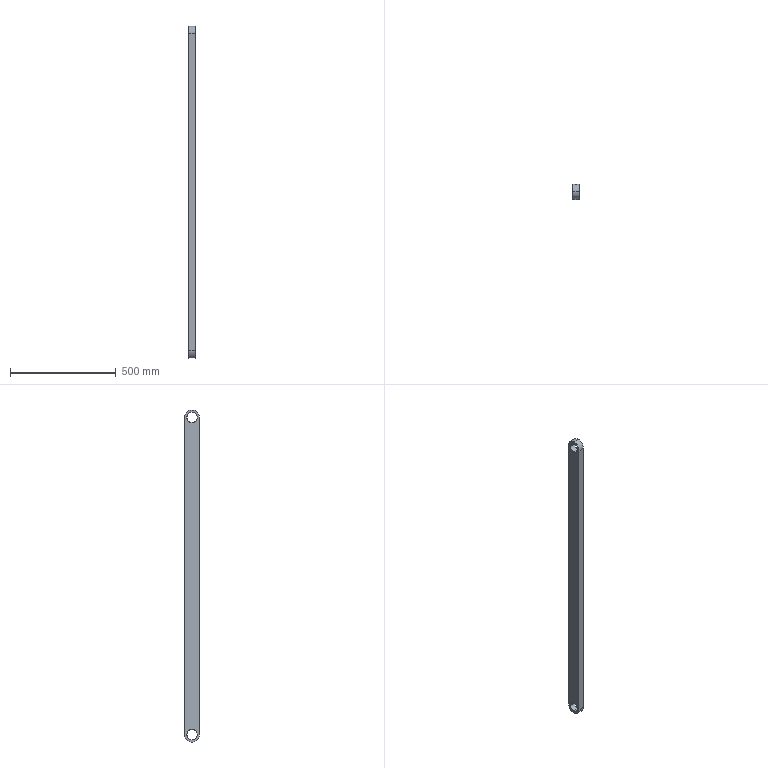Part | SolidWorks | features Chamfer 1, Extrusion 1, HoleWzd 1 | 1 solid | 23 faces | box 30 x 70 x 1570 mm | volume 3155166 mm3 | cylinder 11 | cone 8 | plane 4 | commonest cylinder face diameters 9 x4 48 x4 70 x3
STEP:
#1=CARTESIAN_POINT('',(14.,0.,774.));
#2=VERTEX_POINT('',#1);
#3=CARTESIAN_POINT('',(14.,0.,726.));
#4=VERTEX_POINT('',#3);
#5=CARTESIAN_POINT('',(14.,0.,750.));
#6=DIRECTION('',(1.,0.,0.));
#7=DIRECTION('',(0.,0.,-1.));
#8=AXIS2_PLACEMENT_3D('',#5,#6,#7);
#9=CIRCLE('',#8,24.);
#10=EDGE_CURVE('',#2,#4,#9,.T.);
#11=ORIENTED_EDGE('',*,*,#10,.F.);
#12=CARTESIAN_POINT('',(15.,0.,775.));
#13=VERTEX_POINT('',#12);
#14=CARTESIAN_POINT('',(14.,0.,774.));
#15=DIRECTION('',(0.7071,0.,0.7071));
#16=VECTOR('',#15,1000.);
#17=LINE('',#14,#16);
#18=EDGE_CURVE('',#2,#13,#17,.T.);
#19=ORIENTED_EDGE('',*,*,#18,.T.);
#20=CARTESIAN_POINT('',(15.,0.,725.));
#21=VERTEX_POINT('',#20);
#22=CARTESIAN_POINT('',(15.,0.,750.));
#23=DIRECTION('',(-1.,0.,0.));
#24=DIRECTION('',(0.,0.,-1.));
#25=AXIS2_PLACEMENT_3D('',#22,#23,#24);
#26=CIRCLE('',#25,25.);
#27=EDGE_CURVE('',#21,#13,#26,.T.);
#28=ORIENTED_EDGE('',*,*,#27,.F.);
#29=CARTESIAN_POINT('',(14.,0.,726.));
#30=DIRECTION('',(0.7071,0.,-0.7071));
#31=VECTOR('',#30,1000.);
#32=LINE('',#29,#31);
#33=EDGE_CURVE('',#4,#21,#32,.T.);
#34=ORIENTED_EDGE('',*,*,#33,.F.);
#35=EDGE_LOOP('',(#11,#19,#28,#34));
#36=FACE_OUTER_BOUND('',#35,.T.);
#37=CARTESIAN_POINT('',(14.,0.,750.));
#38=DIRECTION('',(1.,0.,0.));
#39=DIRECTION('',(0.,0.,-1.));
#40=AXIS2_PLACEMENT_3D('',#37,#38,#39);
#41=CONICAL_SURFACE('',#40,24.,0.7854);
#42=ADVANCED_FACE('',(#36),#41,.F.);
#43=CARTESIAN_POINT('',(-14.,0.,726.));
#44=VERTEX_POINT('',#43);
#45=CARTESIAN_POINT('',(-14.,0.,774.));
#46=VERTEX_POINT('',#45);
#47=CARTESIAN_POINT('',(-14.,0.,750.));
#48=DIRECTION('',(-1.,0.,0.));
#49=DIRECTION('',(0.,0.,-1.));
#50=AXIS2_PLACEMENT_3D('',#47,#48,#49);
#51=CIRCLE('',#50,24.);
#52=EDGE_CURVE('',#44,#46,#51,.T.);
#53=ORIENTED_EDGE('',*,*,#52,.F.);
#54=CARTESIAN_POINT('',(-15.,0.,725.));
#55=VERTEX_POINT('',#54);
#56=CARTESIAN_POINT('',(-15.,0.,725.));
#57=DIRECTION('',(-0.7071,0.,-0.7071));
#58=VECTOR('',#57,1000.);
#59=LINE('',#56,#58);
#60=EDGE_CURVE('',#44,#55,#59,.T.);
#61=ORIENTED_EDGE('',*,*,#60,.T.);
#62=CARTESIAN_POINT('',(-15.,0.,775.));
#63=VERTEX_POINT('',#62);
#64=CARTESIAN_POINT('',(-15.,0.,750.));
#65=DIRECTION('',(1.,0.,0.));
#66=DIRECTION('',(0.,0.,-1.));
#67=AXIS2_PLACEMENT_3D('',#64,#65,#66);
#68=CIRCLE('',#67,25.);
#69=EDGE_CURVE('',#63,#55,#68,.T.);
#70=ORIENTED_EDGE('',*,*,#69,.F.);
#71=CARTESIAN_POINT('',(-15.,0.,775.));
#72=DIRECTION('',(-0.7071,0.,0.7071));
#73=VECTOR('',#72,1000.);
#74=LINE('',#71,#73);
#75=EDGE_CURVE('',#46,#63,#74,.T.);
#76=ORIENTED_EDGE('',*,*,#75,.F.);
#77=EDGE_LOOP('',(#53,#61,#70,#76));
#78=FACE_OUTER_BOUND('',#77,.T.);
#79=CARTESIAN_POINT('',(-15.,0.,750.));
#80=DIRECTION('',(-1.,0.,0.));
#81=DIRECTION('',(0.,0.,1.));
#82=AXIS2_PLACEMENT_3D('',#79,#80,#81);
#83=CONICAL_SURFACE('',#82,25.,0.7854);
#84=ADVANCED_FACE('',(#78),#83,.F.);
#85=CARTESIAN_POINT('',(-14.,0.,-774.));
#86=VERTEX_POINT('',#85);
#87=CARTESIAN_POINT('',(-14.,0.,-726.));
#88=VERTEX_POINT('',#87);
#89=CARTESIAN_POINT('',(-14.,0.,-750.));
#90=DIRECTION('',(-1.,0.,0.));
#91=DIRECTION('',(0.,0.,-1.));
#92=AXIS2_PLACEMENT_3D('',#89,#90,#91);
#93=CIRCLE('',#92,24.);
#94=EDGE_CURVE('',#86,#88,#93,.T.);
#95=ORIENTED_EDGE('',*,*,#94,.F.);
#96=CARTESIAN_POINT('',(-15.,0.,-775.));
#97=VERTEX_POINT('',#96);
#98=CARTESIAN_POINT('',(-15.,0.,-775.));
#99=DIRECTION('',(-0.7071,0.,-0.7071));
#100=VECTOR('',#99,1000.);
#101=LINE('',#98,#100);
#102=EDGE_CURVE('',#86,#97,#101,.T.);
#103=ORIENTED_EDGE('',*,*,#102,.T.);
#104=CARTESIAN_POINT('',(-15.,0.,-725.));
#105=VERTEX_POINT('',#104);
#106=CARTESIAN_POINT('',(-15.,0.,-750.));
#107=DIRECTION('',(1.,0.,0.));
#108=DIRECTION('',(0.,0.,-1.));
#109=AXIS2_PLACEMENT_3D('',#106,#107,#108);
#110=CIRCLE('',#109,25.);
#111=EDGE_CURVE('',#105,#97,#110,.T.);
#112=ORIENTED_EDGE('',*,*,#111,.F.);
#113=CARTESIAN_POINT('',(-15.,0.,-725.));
#114=DIRECTION('',(-0.7071,0.,0.7071));
#115=VECTOR('',#114,1000.);
#116=LINE('',#113,#115);
#117=EDGE_CURVE('',#88,#105,#116,.T.);
#118=ORIENTED_EDGE('',*,*,#117,.F.);
#119=EDGE_LOOP('',(#95,#103,#112,#118));
#120=FACE_OUTER_BOUND('',#119,.T.);
#121=CARTESIAN_POINT('',(-15.,0.,-750.));
#122=DIRECTION('',(-1.,0.,0.));
#123=DIRECTION('',(0.,0.,1.));
#124=AXIS2_PLACEMENT_3D('',#121,#122,#123);
#125=CONICAL_SURFACE('',#124,25.,0.7854);
#126=ADVANCED_FACE('',(#120),#125,.F.);
#127=CARTESIAN_POINT('',(14.,0.,-726.));
#128=VERTEX_POINT('',#127);
#129=CARTESIAN_POINT('',(14.,0.,-774.));
#130=VERTEX_POINT('',#129);
#131=CARTESIAN_POINT('',(14.,0.,-750.));
#132=DIRECTION('',(1.,0.,0.));
#133=DIRECTION('',(0.,0.,-1.));
#134=AXIS2_PLACEMENT_3D('',#131,#132,#133);
#135=CIRCLE('',#134,24.);
#136=EDGE_CURVE('',#128,#130,#135,.T.);
#137=ORIENTED_EDGE('',*,*,#136,.F.);
#138=CARTESIAN_POINT('',(15.,0.,-725.));
#139=VERTEX_POINT('',#138);
#140=CARTESIAN_POINT('',(14.,0.,-726.));
#141=DIRECTION('',(0.7071,0.,0.7071));
#142=VECTOR('',#141,1000.);
#143=LINE('',#140,#142);
#144=EDGE_CURVE('',#128,#139,#143,.T.);
#145=ORIENTED_EDGE('',*,*,#144,.T.);
#146=CARTESIAN_POINT('',(15.,0.,-775.));
#147=VERTEX_POINT('',#146);
#148=CARTESIAN_POINT('',(15.,0.,-750.));
#149=DIRECTION('',(-1.,0.,0.));
#150=DIRECTION('',(0.,0.,-1.));
#151=AXIS2_PLACEMENT_3D('',#148,#149,#150);
#152=CIRCLE('',#151,25.);
#153=EDGE_CURVE('',#147,#139,#152,.T.);
#154=ORIENTED_EDGE('',*,*,#153,.F.);
#155=CARTESIAN_POINT('',(14.,0.,-774.));
#156=DIRECTION('',(0.7071,0.,-0.7071));
#157=VECTOR('',#156,1000.);
#158=LINE('',#155,#157);
#159=EDGE_CURVE('',#130,#147,#158,.T.);
#160=ORIENTED_EDGE('',*,*,#159,.F.);
#161=EDGE_LOOP('',(#137,#145,#154,#160));
#162=FACE_OUTER_BOUND('',#161,.T.);
#163=CARTESIAN_POINT('',(14.,0.,-750.));
#164=DIRECTION('',(1.,0.,0.));
#165=DIRECTION('',(0.,0.,-1.));
#166=AXIS2_PLACEMENT_3D('',#163,#164,#165);
#167=CONICAL_SURFACE('',#166,24.,0.7854);
#168=ADVANCED_FACE('',(#162),#167,.F.);
#169=CARTESIAN_POINT('',(0.,23.574,754.5));
#170=VERTEX_POINT('',#169);
#171=CARTESIAN_POINT('',(0.,23.574,745.5));
#172=VERTEX_POINT('',#171);
#173=CARTESIAN_POINT('',(0.,23.574,754.5));
#174=CARTESIAN_POINT('',(-0.298,23.574,754.5));
#175=CARTESIAN_POINT('',(-0.591,23.58,754.471));
#176=CARTESIAN_POINT('',(-1.167,23.601,754.356));
#177=CARTESIAN_POINT('',(-1.453,23.618,754.269));
#178=CARTESIAN_POINT('',(-1.998,23.657,754.043));
#179=CARTESIAN_POINT('',(-2.256,23.681,753.905));
#180=CARTESIAN_POINT('',(-2.745,23.732,753.578));
#181=CARTESIAN_POINT('',(-2.976,23.761,753.388));
#182=CARTESIAN_POINT('',(-3.39,23.816,752.974));
#183=CARTESIAN_POINT('',(-3.576,23.843,752.748));
#184=CARTESIAN_POINT('',(-3.905,23.895,752.256));
#185=CARTESIAN_POINT('',(-4.044,23.918,751.995));
#186=CARTESIAN_POINT('',(-4.269,23.957,751.454));
#187=CARTESIAN_POINT('',(-4.355,23.973,751.17));
#188=CARTESIAN_POINT('',(-4.471,23.995,750.588));
#189=CARTESIAN_POINT('',(-4.5,24.,750.296));
#190=CARTESIAN_POINT('',(-4.5,24.,749.707));
#191=CARTESIAN_POINT('',(-4.471,23.994,749.409));
#192=CARTESIAN_POINT('',(-4.355,23.973,748.831));
#193=CARTESIAN_POINT('',(-4.27,23.958,748.55));
#194=CARTESIAN_POINT('',(-4.044,23.918,748.004));
#195=CARTESIAN_POINT('',(-3.903,23.895,747.742));
#196=CARTESIAN_POINT('',(-3.578,23.844,747.255));
#197=CARTESIAN_POINT('',(-3.391,23.816,747.027));
#198=CARTESIAN_POINT('',(-2.972,23.76,746.609));
#199=CARTESIAN_POINT('',(-2.746,23.732,746.423));
#200=CARTESIAN_POINT('',(-2.259,23.681,746.097));
#201=CARTESIAN_POINT('',(-1.996,23.657,745.956));
#202=CARTESIAN_POINT('',(-1.451,23.617,745.73));
#203=CARTESIAN_POINT('',(-1.171,23.602,745.645));
#204=CARTESIAN_POINT('',(-0.5927,23.58,745.529));
#205=CARTESIAN_POINT('',(-0.294,23.574,745.5));
#206=CARTESIAN_POINT('',(0.,23.574,745.5));
#207=B_SPLINE_CURVE_WITH_KNOTS('',3,(#173,#174,#175,#176,#177,#178,#179,#180,#181,#182,#183,#184,#185,#186,#187,#188,#189,#190,#191,#192,#193,#194,#195,#196,#197,#198,#199,#200,#201,#202,#203,#204,#205,#206),.UNSPECIFIED.,.F.,.F.,(4,2,2,2,2,2,2,2,2,2,2,2,2,2,2,2,4),(0.,0.0008813,0.001763,0.002644,0.003525,0.004406,0.005288,0.006169,0.00705,0.007931,0.008813,0.009694,0.01058,0.01146,0.01234,0.01322,0.0141),.UNSPECIFIED.);
#208=EDGE_CURVE('',#170,#172,#207,.T.);
#209=ORIENTED_EDGE('',*,*,#208,.T.);
#210=CARTESIAN_POINT('',(0.,35.,745.5));
#211=VERTEX_POINT('',#210);
#212=CARTESIAN_POINT('',(0.,35.,745.5));
#213=DIRECTION('',(0.,1.,0.));
#214=VECTOR('',#213,1000.);
#215=LINE('',#212,#214);
#216=EDGE_CURVE('',#172,#211,#215,.T.);
#217=ORIENTED_EDGE('',*,*,#216,.T.);
#218=CARTESIAN_POINT('',(-4.5,35.,750.));
#219=VERTEX_POINT('',#218);
#220=CARTESIAN_POINT('',(0.,35.,750.));
#221=DIRECTION('',(0.,1.,0.));
#222=DIRECTION('',(0.,0.,1.));
#223=AXIS2_PLACEMENT_3D('',#220,#221,#222);
#224=CIRCLE('',#223,4.5);
#225=EDGE_CURVE('',#211,#219,#224,.T.);
#226=ORIENTED_EDGE('',*,*,#225,.T.);
#227=CARTESIAN_POINT('',(0.,34.71,754.5));
#228=VERTEX_POINT('',#227);
#229=CARTESIAN_POINT('',(0.,34.71,754.5));
#230=CARTESIAN_POINT('',(-0.2936,34.71,754.5));
#231=CARTESIAN_POINT('',(-0.5919,34.713,754.471));
#232=CARTESIAN_POINT('',(-1.169,34.728,754.355));
#233=CARTESIAN_POINT('',(-1.449,34.739,754.27));
#234=CARTESIAN_POINT('',(-1.994,34.766,754.045));
#235=CARTESIAN_POINT('',(-2.257,34.782,753.904));
#236=CARTESIAN_POINT('',(-2.744,34.817,753.579));
#237=CARTESIAN_POINT('',(-2.971,34.836,753.393));
#238=CARTESIAN_POINT('',(-3.391,34.874,752.973));
#239=CARTESIAN_POINT('',(-3.577,34.893,752.746));
#240=CARTESIAN_POINT('',(-3.903,34.928,752.26));
#241=CARTESIAN_POINT('',(-4.044,34.944,751.997));
#242=CARTESIAN_POINT('',(-4.269,34.971,751.452));
#243=CARTESIAN_POINT('',(-4.355,34.982,751.172));
#244=CARTESIAN_POINT('',(-4.47,34.996,750.595));
#245=CARTESIAN_POINT('',(-4.5,35.,750.297));
#246=CARTESIAN_POINT('',(-4.5,35.,750.));
#247=B_SPLINE_CURVE_WITH_KNOTS('',3,(#229,#230,#231,#232,#233,#234,#235,#236,#237,#238,#239,#240,#241,#242,#243,#244,#245,#246),.UNSPECIFIED.,.F.,.F.,(4,2,2,2,2,2,2,2,4),(0.007043,0.007923,0.008803,0.009682,0.01056,0.01144,0.01232,0.0132,0.01408),.UNSPECIFIED.);
#248=EDGE_CURVE('',#228,#219,#247,.T.);
#249=ORIENTED_EDGE('',*,*,#248,.F.);
#250=CARTESIAN_POINT('',(0.,35.,754.5));
#251=DIRECTION('',(0.,1.,0.));
#252=VECTOR('',#251,1000.);
#253=LINE('',#250,#252);
#254=EDGE_CURVE('',#170,#228,#253,.T.);
#255=ORIENTED_EDGE('',*,*,#254,.F.);
#256=EDGE_LOOP('',(#209,#217,#226,#249,#255));
#257=FACE_OUTER_BOUND('',#256,.T.);
#258=CARTESIAN_POINT('',(0.,35.,750.));
#259=DIRECTION('',(0.,1.,0.));
#260=DIRECTION('',(0.,0.,1.));
#261=AXIS2_PLACEMENT_3D('',#258,#259,#260);
#262=CYLINDRICAL_SURFACE('',#261,4.5);
#263=ADVANCED_FACE('',(#257),#262,.F.);
#264=CARTESIAN_POINT('',(0.,23.574,-745.5));
#265=VERTEX_POINT('',#264);
#266=CARTESIAN_POINT('',(0.,23.574,-754.5));
#267=VERTEX_POINT('',#266);
#268=CARTESIAN_POINT('',(0.,23.574,-745.5));
#269=CARTESIAN_POINT('',(-0.298,23.574,-745.5));
#270=CARTESIAN_POINT('',(-0.591,23.58,-745.529));
#271=CARTESIAN_POINT('',(-1.167,23.601,-745.644));
#272=CARTESIAN_POINT('',(-1.453,23.618,-745.731));
#273=CARTESIAN_POINT('',(-1.998,23.657,-745.957));
#274=CARTESIAN_POINT('',(-2.256,23.681,-746.095));
#275=CARTESIAN_POINT('',(-2.745,23.732,-746.422));
#276=CARTESIAN_POINT('',(-2.976,23.761,-746.612));
#277=CARTESIAN_POINT('',(-3.39,23.816,-747.026));
#278=CARTESIAN_POINT('',(-3.576,23.843,-747.252));
#279=CARTESIAN_POINT('',(-3.905,23.895,-747.744));
#280=CARTESIAN_POINT('',(-4.044,23.918,-748.005));
#281=CARTESIAN_POINT('',(-4.269,23.957,-748.546));
#282=CARTESIAN_POINT('',(-4.355,23.973,-748.83));
#283=CARTESIAN_POINT('',(-4.471,23.995,-749.412));
#284=CARTESIAN_POINT('',(-4.5,24.,-749.704));
#285=CARTESIAN_POINT('',(-4.5,24.,-750.293));
#286=CARTESIAN_POINT('',(-4.471,23.994,-750.591));
#287=CARTESIAN_POINT('',(-4.355,23.973,-751.169));
#288=CARTESIAN_POINT('',(-4.27,23.958,-751.45));
#289=CARTESIAN_POINT('',(-4.044,23.918,-751.996));
#290=CARTESIAN_POINT('',(-3.903,23.895,-752.258));
#291=CARTESIAN_POINT('',(-3.578,23.844,-752.745));
#292=CARTESIAN_POINT('',(-3.391,23.816,-752.973));
#293=CARTESIAN_POINT('',(-2.972,23.76,-753.391));
#294=CARTESIAN_POINT('',(-2.746,23.732,-753.577));
#295=CARTESIAN_POINT('',(-2.259,23.681,-753.903));
#296=CARTESIAN_POINT('',(-1.996,23.657,-754.044));
#297=CARTESIAN_POINT('',(-1.451,23.617,-754.27));
#298=CARTESIAN_POINT('',(-1.171,23.602,-754.355));
#299=CARTESIAN_POINT('',(-0.5927,23.58,-754.471));
#300=CARTESIAN_POINT('',(-0.294,23.574,-754.5));
#301=CARTESIAN_POINT('',(0.,23.574,-754.5));
#302=B_SPLINE_CURVE_WITH_KNOTS('',3,(#268,#269,#270,#271,#272,#273,#274,#275,#276,#277,#278,#279,#280,#281,#282,#283,#284,#285,#286,#287,#288,#289,#290,#291,#292,#293,#294,#295,#296,#297,#298,#299,#300,#301),.UNSPECIFIED.,.F.,.F.,(4,2,2,2,2,2,2,2,2,2,2,2,2,2,2,2,4),(0.,0.0008813,0.001763,0.002644,0.003525,0.004406,0.005288,0.006169,0.00705,0.007931,0.008813,0.009694,0.01058,0.01146,0.01234,0.01322,0.0141),.UNSPECIFIED.);
#303=EDGE_CURVE('',#265,#267,#302,.T.);
#304=ORIENTED_EDGE('',*,*,#303,.T.);
#305=CARTESIAN_POINT('',(0.,34.71,-754.5));
#306=VERTEX_POINT('',#305);
#307=CARTESIAN_POINT('',(0.,35.,-754.5));
#308=DIRECTION('',(0.,1.,0.));
#309=VECTOR('',#308,1000.);
#310=LINE('',#307,#309);
#311=EDGE_CURVE('',#267,#306,#310,.T.);
#312=ORIENTED_EDGE('',*,*,#311,.T.);
#313=CARTESIAN_POINT('',(-4.5,35.,-750.));
#314=VERTEX_POINT('',#313);
#315=CARTESIAN_POINT('',(-4.5,35.,-750.));
#316=CARTESIAN_POINT('',(-4.5,35.,-750.298));
#317=CARTESIAN_POINT('',(-4.471,34.996,-750.59));
#318=CARTESIAN_POINT('',(-4.356,34.982,-751.166));
#319=CARTESIAN_POINT('',(-4.269,34.971,-751.452));
#320=CARTESIAN_POINT('',(-4.043,34.944,-751.997));
#321=CARTESIAN_POINT('',(-3.905,34.928,-752.256));
#322=CARTESIAN_POINT('',(-3.578,34.893,-752.745));
#323=CARTESIAN_POINT('',(-3.388,34.874,-752.976));
#324=CARTESIAN_POINT('',(-2.973,34.836,-753.391));
#325=CARTESIAN_POINT('',(-2.747,34.817,-753.577));
#326=CARTESIAN_POINT('',(-2.255,34.782,-753.906));
#327=CARTESIAN_POINT('',(-1.993,34.766,-754.045));
#328=CARTESIAN_POINT('',(-1.451,34.739,-754.27));
#329=CARTESIAN_POINT('',(-1.167,34.728,-754.356));
#330=CARTESIAN_POINT('',(-0.5862,34.713,-754.471));
#331=CARTESIAN_POINT('',(-0.2939,34.71,-754.5));
#332=CARTESIAN_POINT('',(0.,34.71,-754.5));
#333=B_SPLINE_CURVE_WITH_KNOTS('',3,(#315,#316,#317,#318,#319,#320,#321,#322,#323,#324,#325,#326,#327,#328,#329,#330,#331,#332),.UNSPECIFIED.,.F.,.F.,(4,2,2,2,2,2,2,2,4),(0.,0.0008804,0.001761,0.002641,0.003522,0.004402,0.005283,0.006163,0.007043),.UNSPECIFIED.);
#334=EDGE_CURVE('',#314,#306,#333,.T.);
#335=ORIENTED_EDGE('',*,*,#334,.F.);
#336=CARTESIAN_POINT('',(0.,35.,-745.5));
#337=VERTEX_POINT('',#336);
#338=CARTESIAN_POINT('',(0.,35.,-750.));
#339=DIRECTION('',(0.,1.,0.));
#340=DIRECTION('',(0.,0.,1.));
#341=AXIS2_PLACEMENT_3D('',#338,#339,#340);
#342=CIRCLE('',#341,4.5);
#343=EDGE_CURVE('',#314,#337,#342,.T.);
#344=ORIENTED_EDGE('',*,*,#343,.T.);
#345=CARTESIAN_POINT('',(0.,35.,-745.5));
#346=DIRECTION('',(0.,1.,0.));
#347=VECTOR('',#346,1000.);
#348=LINE('',#345,#347);
#349=EDGE_CURVE('',#265,#337,#348,.T.);
#350=ORIENTED_EDGE('',*,*,#349,.F.);
#351=EDGE_LOOP('',(#304,#312,#335,#344,#350));
#352=FACE_OUTER_BOUND('',#351,.T.);
#353=CARTESIAN_POINT('',(0.,35.,-750.));
#354=DIRECTION('',(0.,1.,0.));
#355=DIRECTION('',(0.,0.,1.));
#356=AXIS2_PLACEMENT_3D('',#353,#354,#355);
#357=CYLINDRICAL_SURFACE('',#356,4.5);
#358=ADVANCED_FACE('',(#352),#357,.F.);
#359=ORIENTED_EDGE('',*,*,#136,.T.);
#360=CARTESIAN_POINT('',(15.,0.,-774.));
#361=DIRECTION('',(-1.,0.,0.));
#362=VECTOR('',#361,1000.);
#363=LINE('',#360,#362);
#364=EDGE_CURVE('',#130,#86,#363,.T.);
#365=ORIENTED_EDGE('',*,*,#364,.T.);
#366=ORIENTED_EDGE('',*,*,#94,.T.);
#367=CARTESIAN_POINT('',(15.,0.,-726.));
#368=DIRECTION('',(-1.,0.,0.));
#369=VECTOR('',#368,1000.);
#370=LINE('',#367,#369);
#371=EDGE_CURVE('',#128,#88,#370,.T.);
#372=ORIENTED_EDGE('',*,*,#371,.F.);
#373=EDGE_LOOP('',(#359,#365,#366,#372));
#374=FACE_OUTER_BOUND('',#373,.T.);
#375=CARTESIAN_POINT('',(15.,0.,-750.));
#376=DIRECTION('',(-1.,0.,0.));
#377=DIRECTION('',(0.,0.,1.));
#378=AXIS2_PLACEMENT_3D('',#375,#376,#377);
#379=CYLINDRICAL_SURFACE('',#378,24.);
#380=ADVANCED_FACE('',(#374),#379,.F.);
#381=ORIENTED_EDGE('',*,*,#10,.T.);
#382=CARTESIAN_POINT('',(15.,0.,726.));
#383=DIRECTION('',(-1.,0.,0.));
#384=VECTOR('',#383,1000.);
#385=LINE('',#382,#384);
#386=EDGE_CURVE('',#4,#44,#385,.T.);
#387=ORIENTED_EDGE('',*,*,#386,.T.);
#388=ORIENTED_EDGE('',*,*,#52,.T.);
#389=CARTESIAN_POINT('',(15.,0.,774.));
#390=DIRECTION('',(-1.,0.,0.));
#391=VECTOR('',#390,1000.);
#392=LINE('',#389,#391);
#393=EDGE_CURVE('',#2,#46,#392,.T.);
#394=ORIENTED_EDGE('',*,*,#393,.F.);
#395=EDGE_LOOP('',(#381,#387,#388,#394));
#396=FACE_OUTER_BOUND('',#395,.T.);
#397=CARTESIAN_POINT('',(15.,0.,750.));
#398=DIRECTION('',(-1.,0.,0.));
#399=DIRECTION('',(0.,0.,1.));
#400=AXIS2_PLACEMENT_3D('',#397,#398,#399);
#401=CYLINDRICAL_SURFACE('',#400,24.);
#402=ADVANCED_FACE('',(#396),#401,.F.);
#403=CARTESIAN_POINT('',(15.,0.,785.));
#404=VERTEX_POINT('',#403);
#405=CARTESIAN_POINT('',(15.,-35.,750.));
#406=VERTEX_POINT('',#405);
#407=CARTESIAN_POINT('',(15.,0.,750.));
#408=DIRECTION('',(1.,0.,0.));
#409=DIRECTION('',(0.,0.,-1.));
#410=AXIS2_PLACEMENT_3D('',#407,#408,#409);
#411=CIRCLE('',#410,35.);
#412=EDGE_CURVE('',#404,#406,#411,.T.);
#413=ORIENTED_EDGE('',*,*,#412,.F.);
#414=CARTESIAN_POINT('',(-15.,0.,785.));
#415=VERTEX_POINT('',#414);
#416=CARTESIAN_POINT('',(15.,0.,785.));
#417=DIRECTION('',(-1.,0.,0.));
#418=VECTOR('',#417,1000.);
#419=LINE('',#416,#418);
#420=EDGE_CURVE('',#404,#415,#419,.T.);
#421=ORIENTED_EDGE('',*,*,#420,.T.);
#422=CARTESIAN_POINT('',(-15.,-35.,750.));
#423=VERTEX_POINT('',#422);
#424=CARTESIAN_POINT('',(-15.,0.,750.));
#425=DIRECTION('',(1.,0.,0.));
#426=DIRECTION('',(0.,0.,-1.));
#427=AXIS2_PLACEMENT_3D('',#424,#425,#426);
#428=CIRCLE('',#427,35.);
#429=EDGE_CURVE('',#415,#423,#428,.T.);
#430=ORIENTED_EDGE('',*,*,#429,.T.);
#431=CARTESIAN_POINT('',(15.,-35.,750.));
#432=DIRECTION('',(-1.,0.,0.));
#433=VECTOR('',#432,1000.);
#434=LINE('',#431,#433);
#435=EDGE_CURVE('',#406,#423,#434,.T.);
#436=ORIENTED_EDGE('',*,*,#435,.F.);
#437=EDGE_LOOP('',(#413,#421,#430,#436));
#438=FACE_OUTER_BOUND('',#437,.T.);
#439=CARTESIAN_POINT('',(15.,0.,750.));
#440=DIRECTION('',(-1.,0.,0.));
#441=DIRECTION('',(0.,0.,1.));
#442=AXIS2_PLACEMENT_3D('',#439,#440,#441);
#443=CYLINDRICAL_SURFACE('',#442,35.);
#444=ADVANCED_FACE('',(#438),#443,.T.);
#445=ORIENTED_EDGE('',*,*,#153,.T.);
#446=CARTESIAN_POINT('',(15.,0.,-750.));
#447=DIRECTION('',(-1.,0.,0.));
#448=DIRECTION('',(0.,0.,-1.));
#449=AXIS2_PLACEMENT_3D('',#446,#447,#448);
#450=CIRCLE('',#449,25.);
#451=EDGE_CURVE('',#139,#147,#450,.T.);
#452=ORIENTED_EDGE('',*,*,#451,.T.);
#453=EDGE_LOOP('',(#445,#452));
#454=FACE_BOUND('',#453,.T.);
#455=ORIENTED_EDGE('',*,*,#27,.T.);
#456=CARTESIAN_POINT('',(15.,0.,750.));
#457=DIRECTION('',(-1.,0.,0.));
#458=DIRECTION('',(0.,0.,-1.));
#459=AXIS2_PLACEMENT_3D('',#456,#457,#458);
#460=CIRCLE('',#459,25.);
#461=EDGE_CURVE('',#13,#21,#460,.T.);
#462=ORIENTED_EDGE('',*,*,#461,.T.);
#463=EDGE_LOOP('',(#455,#462));
#464=FACE_BOUND('',#463,.T.);
#465=CARTESIAN_POINT('',(15.,35.,750.));
#466=VERTEX_POINT('',#465);
#467=CARTESIAN_POINT('',(15.,0.,750.));
#468=DIRECTION('',(1.,0.,0.));
#469=DIRECTION('',(0.,0.,-1.));
#470=AXIS2_PLACEMENT_3D('',#467,#468,#469);
#471=CIRCLE('',#470,35.);
#472=EDGE_CURVE('',#466,#404,#471,.T.);
#473=ORIENTED_EDGE('',*,*,#472,.T.);
#474=ORIENTED_EDGE('',*,*,#412,.T.);
#475=CARTESIAN_POINT('',(15.,-35.,-750.));
#476=VERTEX_POINT('',#475);
#477=CARTESIAN_POINT('',(15.,-35.,750.));
#478=DIRECTION('',(0.,0.,-1.));
#479=VECTOR('',#478,1000.);
#480=LINE('',#477,#479);
#481=EDGE_CURVE('',#406,#476,#480,.T.);
#482=ORIENTED_EDGE('',*,*,#481,.T.);
#483=CARTESIAN_POINT('',(15.,35.,-750.));
#484=VERTEX_POINT('',#483);
#485=CARTESIAN_POINT('',(15.,0.,-750.));
#486=DIRECTION('',(1.,0.,0.));
#487=DIRECTION('',(0.,0.,1.));
#488=AXIS2_PLACEMENT_3D('',#485,#486,#487);
#489=CIRCLE('',#488,35.);
#490=EDGE_CURVE('',#476,#484,#489,.T.);
#491=ORIENTED_EDGE('',*,*,#490,.T.);
#492=CARTESIAN_POINT('',(15.,35.,750.));
#493=DIRECTION('',(0.,0.,1.));
#494=VECTOR('',#493,1000.);
#495=LINE('',#492,#494);
#496=EDGE_CURVE('',#484,#466,#495,.T.);
#497=ORIENTED_EDGE('',*,*,#496,.T.);
#498=EDGE_LOOP('',(#473,#474,#482,#491,#497));
#499=FACE_OUTER_BOUND('',#498,.T.);
#500=CARTESIAN_POINT('',(15.,0.,750.));
#501=DIRECTION('',(1.,0.,0.));
#502=DIRECTION('',(0.,0.,-1.));
#503=AXIS2_PLACEMENT_3D('',#500,#501,#502);
#504=PLANE('',#503);
#505=ADVANCED_FACE('',(#454,#464,#499),#504,.T.);
#506=ORIENTED_EDGE('',*,*,#111,.T.);
#507=CARTESIAN_POINT('',(-15.,0.,-750.));
#508=DIRECTION('',(1.,0.,0.));
#509=DIRECTION('',(0.,0.,-1.));
#510=AXIS2_PLACEMENT_3D('',#507,#508,#509);
#511=CIRCLE('',#510,25.);
#512=EDGE_CURVE('',#97,#105,#511,.T.);
#513=ORIENTED_EDGE('',*,*,#512,.T.);
#514=EDGE_LOOP('',(#506,#513));
#515=FACE_BOUND('',#514,.T.);
#516=ORIENTED_EDGE('',*,*,#69,.T.);
#517=CARTESIAN_POINT('',(-15.,0.,750.));
#518=DIRECTION('',(1.,0.,0.));
#519=DIRECTION('',(0.,0.,-1.));
#520=AXIS2_PLACEMENT_3D('',#517,#518,#519);
#521=CIRCLE('',#520,25.);
#522=EDGE_CURVE('',#55,#63,#521,.T.);
#523=ORIENTED_EDGE('',*,*,#522,.T.);
#524=EDGE_LOOP('',(#516,#523));
#525=FACE_BOUND('',#524,.T.);
#526=CARTESIAN_POINT('',(-15.,35.,750.));
#527=VERTEX_POINT('',#526);
#528=CARTESIAN_POINT('',(-15.,0.,750.));
#529=DIRECTION('',(1.,0.,0.));
#530=DIRECTION('',(0.,0.,-1.));
#531=AXIS2_PLACEMENT_3D('',#528,#529,#530);
#532=CIRCLE('',#531,35.);
#533=EDGE_CURVE('',#527,#415,#532,.T.);
#534=ORIENTED_EDGE('',*,*,#533,.F.);
#535=CARTESIAN_POINT('',(-15.,35.,-750.));
#536=VERTEX_POINT('',#535);
#537=CARTESIAN_POINT('',(-15.,35.,750.));
#538=DIRECTION('',(0.,0.,1.));
#539=VECTOR('',#538,1000.);
#540=LINE('',#537,#539);
#541=EDGE_CURVE('',#536,#527,#540,.T.);
#542=ORIENTED_EDGE('',*,*,#541,.F.);
#543=CARTESIAN_POINT('',(-15.,-35.,-750.));
#544=VERTEX_POINT('',#543);
#545=CARTESIAN_POINT('',(-15.,0.,-750.));
#546=DIRECTION('',(1.,0.,0.));
#547=DIRECTION('',(0.,0.,1.));
#548=AXIS2_PLACEMENT_3D('',#545,#546,#547);
#549=CIRCLE('',#548,35.);
#550=EDGE_CURVE('',#544,#536,#549,.T.);
#551=ORIENTED_EDGE('',*,*,#550,.F.);
#552=CARTESIAN_POINT('',(-15.,-35.,750.));
#553=DIRECTION('',(0.,0.,-1.));
#554=VECTOR('',#553,1000.);
#555=LINE('',#552,#554);
#556=EDGE_CURVE('',#423,#544,#555,.T.);
#557=ORIENTED_EDGE('',*,*,#556,.F.);
#558=ORIENTED_EDGE('',*,*,#429,.F.);
#559=EDGE_LOOP('',(#534,#542,#551,#557,#558));
#560=FACE_OUTER_BOUND('',#559,.T.);
#561=CARTESIAN_POINT('',(-15.,0.,750.));
#562=DIRECTION('',(1.,0.,0.));
#563=DIRECTION('',(0.,0.,-1.));
#564=AXIS2_PLACEMENT_3D('',#561,#562,#563);
#565=PLANE('',#564);
#566=ADVANCED_FACE('',(#515,#525,#560),#565,.F.);
#567=ORIENTED_EDGE('',*,*,#420,.F.);
#568=ORIENTED_EDGE('',*,*,#472,.F.);
#569=CARTESIAN_POINT('',(4.5,35.,750.));
#570=VERTEX_POINT('',#569);
#571=CARTESIAN_POINT('',(15.,35.,750.));
#572=DIRECTION('',(-1.,0.,0.));
#573=VECTOR('',#572,1000.);
#574=LINE('',#571,#573);
#575=EDGE_CURVE('',#466,#570,#574,.T.);
#576=ORIENTED_EDGE('',*,*,#575,.T.);
#577=CARTESIAN_POINT('',(4.5,35.,750.));
#578=CARTESIAN_POINT('',(4.5,35.,750.298));
#579=CARTESIAN_POINT('',(4.471,34.996,750.59));
#580=CARTESIAN_POINT('',(4.356,34.982,751.166));
#581=CARTESIAN_POINT('',(4.269,34.971,751.452));
#582=CARTESIAN_POINT('',(4.043,34.944,751.997));
#583=CARTESIAN_POINT('',(3.905,34.928,752.256));
#584=CARTESIAN_POINT('',(3.578,34.893,752.745));
#585=CARTESIAN_POINT('',(3.388,34.874,752.976));
#586=CARTESIAN_POINT('',(2.973,34.836,753.391));
#587=CARTESIAN_POINT('',(2.747,34.817,753.577));
#588=CARTESIAN_POINT('',(2.255,34.782,753.906));
#589=CARTESIAN_POINT('',(1.993,34.766,754.045));
#590=CARTESIAN_POINT('',(1.451,34.739,754.27));
#591=CARTESIAN_POINT('',(1.167,34.728,754.356));
#592=CARTESIAN_POINT('',(0.5862,34.713,754.471));
#593=CARTESIAN_POINT('',(0.2939,34.71,754.5));
#594=CARTESIAN_POINT('',(0.,34.71,754.5));
#595=B_SPLINE_CURVE_WITH_KNOTS('',3,(#577,#578,#579,#580,#581,#582,#583,#584,#585,#586,#587,#588,#589,#590,#591,#592,#593,#594),.UNSPECIFIED.,.F.,.F.,(4,2,2,2,2,2,2,2,4),(0.,0.0008804,0.001761,0.002641,0.003522,0.004402,0.005283,0.006163,0.007043),.UNSPECIFIED.);
#596=EDGE_CURVE('',#570,#228,#595,.T.);
#597=ORIENTED_EDGE('',*,*,#596,.T.);
#598=ORIENTED_EDGE('',*,*,#248,.T.);
#599=CARTESIAN_POINT('',(15.,35.,750.));
#600=DIRECTION('',(-1.,0.,0.));
#601=VECTOR('',#600,1000.);
#602=LINE('',#599,#601);
#603=EDGE_CURVE('',#219,#527,#602,.T.);
#604=ORIENTED_EDGE('',*,*,#603,.T.);
#605=ORIENTED_EDGE('',*,*,#533,.T.);
#606=EDGE_LOOP('',(#567,#568,#576,#597,#598,#604,#605));
#607=FACE_OUTER_BOUND('',#606,.T.);
#608=CARTESIAN_POINT('',(15.,0.,750.));
#609=DIRECTION('',(-1.,0.,0.));
#610=DIRECTION('',(0.,0.,1.));
#611=AXIS2_PLACEMENT_3D('',#608,#609,#610);
#612=CYLINDRICAL_SURFACE('',#611,35.);
#613=ADVANCED_FACE('',(#607),#612,.T.);
#614=ORIENTED_EDGE('',*,*,#556,.T.);
#615=CARTESIAN_POINT('',(15.,-35.,-750.));
#616=DIRECTION('',(-1.,0.,0.));
#617=VECTOR('',#616,1000.);
#618=LINE('',#615,#617);
#619=EDGE_CURVE('',#476,#544,#618,.T.);
#620=ORIENTED_EDGE('',*,*,#619,.F.);
#621=ORIENTED_EDGE('',*,*,#481,.F.);
#622=ORIENTED_EDGE('',*,*,#435,.T.);
#623=EDGE_LOOP('',(#614,#620,#621,#622));
#624=FACE_OUTER_BOUND('',#623,.T.);
#625=CARTESIAN_POINT('',(15.,-35.,750.));
#626=DIRECTION('',(0.,1.,0.));
#627=DIRECTION('',(0.,0.,1.));
#628=AXIS2_PLACEMENT_3D('',#625,#626,#627);
#629=PLANE('',#628);
#630=ADVANCED_FACE('',(#624),#629,.F.);
#631=CARTESIAN_POINT('',(15.,35.,-750.));
#632=DIRECTION('',(-1.,0.,0.));
#633=VECTOR('',#632,1000.);
#634=LINE('',#631,#633);
#635=EDGE_CURVE('',#314,#536,#634,.T.);
#636=ORIENTED_EDGE('',*,*,#635,.F.);
#637=ORIENTED_EDGE('',*,*,#334,.T.);
#638=CARTESIAN_POINT('',(4.5,35.,-750.));
#639=VERTEX_POINT('',#638);
#640=CARTESIAN_POINT('',(0.,34.71,-754.5));
#641=CARTESIAN_POINT('',(0.2936,34.71,-754.5));
#642=CARTESIAN_POINT('',(0.5919,34.713,-754.471));
#643=CARTESIAN_POINT('',(1.169,34.728,-754.355));
#644=CARTESIAN_POINT('',(1.449,34.739,-754.27));
#645=CARTESIAN_POINT('',(1.994,34.766,-754.045));
#646=CARTESIAN_POINT('',(2.257,34.782,-753.904));
#647=CARTESIAN_POINT('',(2.744,34.817,-753.579));
#648=CARTESIAN_POINT('',(2.971,34.836,-753.393));
#649=CARTESIAN_POINT('',(3.391,34.874,-752.973));
#650=CARTESIAN_POINT('',(3.577,34.893,-752.746));
#651=CARTESIAN_POINT('',(3.903,34.928,-752.26));
#652=CARTESIAN_POINT('',(4.044,34.944,-751.997));
#653=CARTESIAN_POINT('',(4.269,34.971,-751.452));
#654=CARTESIAN_POINT('',(4.355,34.982,-751.172));
#655=CARTESIAN_POINT('',(4.47,34.996,-750.595));
#656=CARTESIAN_POINT('',(4.5,35.,-750.297));
#657=CARTESIAN_POINT('',(4.5,35.,-750.));
#658=B_SPLINE_CURVE_WITH_KNOTS('',3,(#640,#641,#642,#643,#644,#645,#646,#647,#648,#649,#650,#651,#652,#653,#654,#655,#656,#657),.UNSPECIFIED.,.F.,.F.,(4,2,2,2,2,2,2,2,4),(0.007043,0.007923,0.008803,0.009682,0.01056,0.01144,0.01232,0.0132,0.01408),.UNSPECIFIED.);
#659=EDGE_CURVE('',#306,#639,#658,.T.);
#660=ORIENTED_EDGE('',*,*,#659,.T.);
#661=CARTESIAN_POINT('',(15.,35.,-750.));
#662=DIRECTION('',(-1.,0.,0.));
#663=VECTOR('',#662,1000.);
#664=LINE('',#661,#663);
#665=EDGE_CURVE('',#484,#639,#664,.T.);
#666=ORIENTED_EDGE('',*,*,#665,.F.);
#667=ORIENTED_EDGE('',*,*,#490,.F.);
#668=ORIENTED_EDGE('',*,*,#619,.T.);
#669=ORIENTED_EDGE('',*,*,#550,.T.);
#670=EDGE_LOOP('',(#636,#637,#660,#666,#667,#668,#669));
#671=FACE_OUTER_BOUND('',#670,.T.);
#672=CARTESIAN_POINT('',(15.,0.,-750.));
#673=DIRECTION('',(-1.,0.,0.));
#674=DIRECTION('',(0.,0.,1.));
#675=AXIS2_PLACEMENT_3D('',#672,#673,#674);
#676=CYLINDRICAL_SURFACE('',#675,35.);
#677=ADVANCED_FACE('',(#671),#676,.T.);
#678=ORIENTED_EDGE('',*,*,#603,.F.);
#679=ORIENTED_EDGE('',*,*,#225,.F.);
#680=CARTESIAN_POINT('',(0.,35.,750.));
#681=DIRECTION('',(0.,1.,0.));
#682=DIRECTION('',(0.,0.,1.));
#683=AXIS2_PLACEMENT_3D('',#680,#681,#682);
#684=CIRCLE('',#683,4.5);
#685=EDGE_CURVE('',#570,#211,#684,.T.);
#686=ORIENTED_EDGE('',*,*,#685,.F.);
#687=ORIENTED_EDGE('',*,*,#575,.F.);
#688=ORIENTED_EDGE('',*,*,#496,.F.);
#689=ORIENTED_EDGE('',*,*,#665,.T.);
#690=CARTESIAN_POINT('',(0.,35.,-750.));
#691=DIRECTION('',(0.,1.,0.));
#692=DIRECTION('',(0.,0.,1.));
#693=AXIS2_PLACEMENT_3D('',#690,#691,#692);
#694=CIRCLE('',#693,4.5);
#695=EDGE_CURVE('',#337,#639,#694,.T.);
#696=ORIENTED_EDGE('',*,*,#695,.F.);
#697=ORIENTED_EDGE('',*,*,#343,.F.);
#698=ORIENTED_EDGE('',*,*,#635,.T.);
#699=ORIENTED_EDGE('',*,*,#541,.T.);
#700=EDGE_LOOP('',(#678,#679,#686,#687,#688,#689,#696,#697,#698,#699));
#701=FACE_OUTER_BOUND('',#700,.T.);
#702=CARTESIAN_POINT('',(15.,35.,750.));
#703=DIRECTION('',(0.,-1.,0.));
#704=DIRECTION('',(0.,0.,-1.));
#705=AXIS2_PLACEMENT_3D('',#702,#703,#704);
#706=PLANE('',#705);
#707=ADVANCED_FACE('',(#701),#706,.F.);
#708=ORIENTED_EDGE('',*,*,#386,.F.);
#709=CARTESIAN_POINT('',(14.,0.,750.));
#710=DIRECTION('',(1.,0.,0.));
#711=DIRECTION('',(0.,0.,-1.));
#712=AXIS2_PLACEMENT_3D('',#709,#710,#711);
#713=CIRCLE('',#712,24.);
#714=EDGE_CURVE('',#4,#2,#713,.T.);
#715=ORIENTED_EDGE('',*,*,#714,.T.);
#716=ORIENTED_EDGE('',*,*,#393,.T.);
#717=CARTESIAN_POINT('',(-14.,0.,750.));
#718=DIRECTION('',(-1.,0.,0.));
#719=DIRECTION('',(0.,0.,-1.));
#720=AXIS2_PLACEMENT_3D('',#717,#718,#719);
#721=CIRCLE('',#720,24.);
#722=EDGE_CURVE('',#46,#44,#721,.T.);
#723=ORIENTED_EDGE('',*,*,#722,.T.);
#724=EDGE_LOOP('',(#708,#715,#716,#723));
#725=FACE_OUTER_BOUND('',#724,.T.);
#726=ORIENTED_EDGE('',*,*,#208,.F.);
#727=CARTESIAN_POINT('',(0.,23.574,745.5));
#728=CARTESIAN_POINT('',(0.294,23.574,745.5));
#729=CARTESIAN_POINT('',(0.5866,23.58,745.529));
#730=CARTESIAN_POINT('',(1.169,23.602,745.644));
#731=CARTESIAN_POINT('',(1.452,23.617,745.731));
#732=CARTESIAN_POINT('',(1.994,23.657,745.955));
#733=CARTESIAN_POINT('',(2.256,23.681,746.095));
#734=CARTESIAN_POINT('',(2.746,23.733,746.423));
#735=CARTESIAN_POINT('',(2.973,23.76,746.609));
#736=CARTESIAN_POINT('',(3.388,23.816,747.023));
#737=CARTESIAN_POINT('',(3.577,23.844,747.254));
#738=CARTESIAN_POINT('',(3.903,23.895,747.742));
#739=CARTESIAN_POINT('',(4.042,23.918,748.));
#740=CARTESIAN_POINT('',(4.269,23.957,748.545));
#741=CARTESIAN_POINT('',(4.355,23.973,748.83));
#742=CARTESIAN_POINT('',(4.47,23.994,749.406));
#743=CARTESIAN_POINT('',(4.5,24.,749.7));
#744=CARTESIAN_POINT('',(4.5,24.,750.295));
#745=CARTESIAN_POINT('',(4.471,23.995,750.587));
#746=CARTESIAN_POINT('',(4.357,23.973,751.164));
#747=CARTESIAN_POINT('',(4.27,23.958,751.451));
#748=CARTESIAN_POINT('',(4.045,23.919,751.994));
#749=CARTESIAN_POINT('',(3.907,23.895,752.253));
#750=CARTESIAN_POINT('',(3.58,23.844,752.743));
#751=CARTESIAN_POINT('',(3.391,23.816,752.973));
#752=CARTESIAN_POINT('',(2.977,23.761,753.387));
#753=CARTESIAN_POINT('',(2.751,23.733,753.573));
#754=CARTESIAN_POINT('',(2.258,23.681,753.904));
#755=CARTESIAN_POINT('',(1.999,23.657,754.042));
#756=CARTESIAN_POINT('',(1.458,23.618,754.267));
#757=CARTESIAN_POINT('',(1.173,23.602,754.354));
#758=CARTESIAN_POINT('',(0.5921,23.58,754.471));
#759=CARTESIAN_POINT('',(0.298,23.574,754.5));
#760=CARTESIAN_POINT('',(0.,23.574,754.5));
#761=B_SPLINE_CURVE_WITH_KNOTS('',3,(#727,#728,#729,#730,#731,#732,#733,#734,#735,#736,#737,#738,#739,#740,#741,#742,#743,#744,#745,#746,#747,#748,#749,#750,#751,#752,#753,#754,#755,#756,#757,#758,#759,#760),.UNSPECIFIED.,.F.,.F.,(4,2,2,2,2,2,2,2,2,2,2,2,2,2,2,2,4),(0.0141,0.01498,0.01586,0.01674,0.01762,0.01851,0.01939,0.02027,0.02115,0.02203,0.02291,0.02379,0.02467,0.02555,0.02643,0.02732,0.0282),.UNSPECIFIED.);
#762=EDGE_CURVE('',#172,#170,#761,.T.);
#763=ORIENTED_EDGE('',*,*,#762,.F.);
#764=EDGE_LOOP('',(#726,#763));
#765=FACE_BOUND('',#764,.T.);
#766=CARTESIAN_POINT('',(15.,0.,750.));
#767=DIRECTION('',(-1.,0.,0.));
#768=DIRECTION('',(0.,0.,1.));
#769=AXIS2_PLACEMENT_3D('',#766,#767,#768);
#770=CYLINDRICAL_SURFACE('',#769,24.);
#771=ADVANCED_FACE('',(#725,#765),#770,.F.);
#772=ORIENTED_EDGE('',*,*,#364,.F.);
#773=CARTESIAN_POINT('',(14.,0.,-750.));
#774=DIRECTION('',(1.,0.,0.));
#775=DIRECTION('',(0.,0.,-1.));
#776=AXIS2_PLACEMENT_3D('',#773,#774,#775);
#777=CIRCLE('',#776,24.);
#778=EDGE_CURVE('',#130,#128,#777,.T.);
#779=ORIENTED_EDGE('',*,*,#778,.T.);
#780=ORIENTED_EDGE('',*,*,#371,.T.);
#781=CARTESIAN_POINT('',(-14.,0.,-750.));
#782=DIRECTION('',(-1.,0.,0.));
#783=DIRECTION('',(0.,0.,-1.));
#784=AXIS2_PLACEMENT_3D('',#781,#782,#783);
#785=CIRCLE('',#784,24.);
#786=EDGE_CURVE('',#88,#86,#785,.T.);
#787=ORIENTED_EDGE('',*,*,#786,.T.);
#788=EDGE_LOOP('',(#772,#779,#780,#787));
#789=FACE_OUTER_BOUND('',#788,.T.);
#790=ORIENTED_EDGE('',*,*,#303,.F.);
#791=CARTESIAN_POINT('',(0.,23.574,-754.5));
#792=CARTESIAN_POINT('',(0.294,23.574,-754.5));
#793=CARTESIAN_POINT('',(0.5866,23.58,-754.471));
#794=CARTESIAN_POINT('',(1.169,23.602,-754.356));
#795=CARTESIAN_POINT('',(1.452,23.617,-754.269));
#796=CARTESIAN_POINT('',(1.994,23.657,-754.045));
#797=CARTESIAN_POINT('',(2.256,23.681,-753.905));
#798=CARTESIAN_POINT('',(2.746,23.733,-753.577));
#799=CARTESIAN_POINT('',(2.973,23.76,-753.391));
#800=CARTESIAN_POINT('',(3.388,23.816,-752.977));
#801=CARTESIAN_POINT('',(3.577,23.844,-752.746));
#802=CARTESIAN_POINT('',(3.903,23.895,-752.258));
#803=CARTESIAN_POINT('',(4.042,23.918,-752.));
#804=CARTESIAN_POINT('',(4.269,23.957,-751.455));
#805=CARTESIAN_POINT('',(4.355,23.973,-751.17));
#806=CARTESIAN_POINT('',(4.47,23.994,-750.594));
#807=CARTESIAN_POINT('',(4.5,24.,-750.3));
#808=CARTESIAN_POINT('',(4.5,24.,-749.705));
#809=CARTESIAN_POINT('',(4.471,23.995,-749.413));
#810=CARTESIAN_POINT('',(4.357,23.973,-748.836));
#811=CARTESIAN_POINT('',(4.27,23.958,-748.549));
#812=CARTESIAN_POINT('',(4.045,23.919,-748.006));
#813=CARTESIAN_POINT('',(3.907,23.895,-747.747));
#814=CARTESIAN_POINT('',(3.58,23.844,-747.257));
#815=CARTESIAN_POINT('',(3.391,23.816,-747.027));
#816=CARTESIAN_POINT('',(2.977,23.761,-746.613));
#817=CARTESIAN_POINT('',(2.751,23.733,-746.427));
#818=CARTESIAN_POINT('',(2.258,23.681,-746.096));
#819=CARTESIAN_POINT('',(1.999,23.657,-745.958));
#820=CARTESIAN_POINT('',(1.458,23.618,-745.733));
#821=CARTESIAN_POINT('',(1.173,23.602,-745.646));
#822=CARTESIAN_POINT('',(0.5921,23.58,-745.529));
#823=CARTESIAN_POINT('',(0.298,23.574,-745.5));
#824=CARTESIAN_POINT('',(0.,23.574,-745.5));
#825=B_SPLINE_CURVE_WITH_KNOTS('',3,(#791,#792,#793,#794,#795,#796,#797,#798,#799,#800,#801,#802,#803,#804,#805,#806,#807,#808,#809,#810,#811,#812,#813,#814,#815,#816,#817,#818,#819,#820,#821,#822,#823,#824),.UNSPECIFIED.,.F.,.F.,(4,2,2,2,2,2,2,2,2,2,2,2,2,2,2,2,4),(0.0141,0.01498,0.01586,0.01674,0.01762,0.01851,0.01939,0.02027,0.02115,0.02203,0.02291,0.02379,0.02467,0.02555,0.02643,0.02732,0.0282),.UNSPECIFIED.);
#826=EDGE_CURVE('',#267,#265,#825,.T.);
#827=ORIENTED_EDGE('',*,*,#826,.F.);
#828=EDGE_LOOP('',(#790,#827));
#829=FACE_BOUND('',#828,.T.);
#830=CARTESIAN_POINT('',(15.,0.,-750.));
#831=DIRECTION('',(-1.,0.,0.));
#832=DIRECTION('',(0.,0.,1.));
#833=AXIS2_PLACEMENT_3D('',#830,#831,#832);
#834=CYLINDRICAL_SURFACE('',#833,24.);
#835=ADVANCED_FACE('',(#789,#829),#834,.F.);
#836=ORIENTED_EDGE('',*,*,#311,.F.);
#837=ORIENTED_EDGE('',*,*,#826,.T.);
#838=ORIENTED_EDGE('',*,*,#349,.T.);
#839=ORIENTED_EDGE('',*,*,#695,.T.);
#840=ORIENTED_EDGE('',*,*,#659,.F.);
#841=EDGE_LOOP('',(#836,#837,#838,#839,#840));
#842=FACE_OUTER_BOUND('',#841,.T.);
#843=CARTESIAN_POINT('',(0.,35.,-750.));
#844=DIRECTION('',(0.,1.,0.));
#845=DIRECTION('',(0.,0.,1.));
#846=AXIS2_PLACEMENT_3D('',#843,#844,#845);
#847=CYLINDRICAL_SURFACE('',#846,4.5);
#848=ADVANCED_FACE('',(#842),#847,.F.);
#849=ORIENTED_EDGE('',*,*,#216,.F.);
#850=ORIENTED_EDGE('',*,*,#762,.T.);
#851=ORIENTED_EDGE('',*,*,#254,.T.);
#852=ORIENTED_EDGE('',*,*,#596,.F.);
#853=ORIENTED_EDGE('',*,*,#685,.T.);
#854=EDGE_LOOP('',(#849,#850,#851,#852,#853));
#855=FACE_OUTER_BOUND('',#854,.T.);
#856=CARTESIAN_POINT('',(0.,35.,750.));
#857=DIRECTION('',(0.,1.,0.));
#858=DIRECTION('',(0.,0.,1.));
#859=AXIS2_PLACEMENT_3D('',#856,#857,#858);
#860=CYLINDRICAL_SURFACE('',#859,4.5);
#861=ADVANCED_FACE('',(#855),#860,.F.);
#862=ORIENTED_EDGE('',*,*,#144,.F.);
#863=ORIENTED_EDGE('',*,*,#778,.F.);
#864=ORIENTED_EDGE('',*,*,#159,.T.);
#865=ORIENTED_EDGE('',*,*,#451,.F.);
#866=EDGE_LOOP('',(#862,#863,#864,#865));
#867=FACE_OUTER_BOUND('',#866,.T.);
#868=CARTESIAN_POINT('',(14.,0.,-750.));
#869=DIRECTION('',(1.,0.,0.));
#870=DIRECTION('',(0.,0.,-1.));
#871=AXIS2_PLACEMENT_3D('',#868,#869,#870);
#872=CONICAL_SURFACE('',#871,24.,0.7854);
#873=ADVANCED_FACE('',(#867),#872,.F.);
#874=ORIENTED_EDGE('',*,*,#102,.F.);
#875=ORIENTED_EDGE('',*,*,#786,.F.);
#876=ORIENTED_EDGE('',*,*,#117,.T.);
#877=ORIENTED_EDGE('',*,*,#512,.F.);
#878=EDGE_LOOP('',(#874,#875,#876,#877));
#879=FACE_OUTER_BOUND('',#878,.T.);
#880=CARTESIAN_POINT('',(-15.,0.,-750.));
#881=DIRECTION('',(-1.,0.,0.));
#882=DIRECTION('',(0.,0.,1.));
#883=AXIS2_PLACEMENT_3D('',#880,#881,#882);
#884=CONICAL_SURFACE('',#883,25.,0.7854);
#885=ADVANCED_FACE('',(#879),#884,.F.);
#886=ORIENTED_EDGE('',*,*,#60,.F.);
#887=ORIENTED_EDGE('',*,*,#722,.F.);
#888=ORIENTED_EDGE('',*,*,#75,.T.);
#889=ORIENTED_EDGE('',*,*,#522,.F.);
#890=EDGE_LOOP('',(#886,#887,#888,#889));
#891=FACE_OUTER_BOUND('',#890,.T.);
#892=CARTESIAN_POINT('',(-15.,0.,750.));
#893=DIRECTION('',(-1.,0.,0.));
#894=DIRECTION('',(0.,0.,1.));
#895=AXIS2_PLACEMENT_3D('',#892,#893,#894);
#896=CONICAL_SURFACE('',#895,25.,0.7854);
#897=ADVANCED_FACE('',(#891),#896,.F.);
#898=ORIENTED_EDGE('',*,*,#18,.F.);
#899=ORIENTED_EDGE('',*,*,#714,.F.);
#900=ORIENTED_EDGE('',*,*,#33,.T.);
#901=ORIENTED_EDGE('',*,*,#461,.F.);
#902=EDGE_LOOP('',(#898,#899,#900,#901));
#903=FACE_OUTER_BOUND('',#902,.T.);
#904=CARTESIAN_POINT('',(14.,0.,750.));
#905=DIRECTION('',(1.,0.,0.));
#906=DIRECTION('',(0.,0.,-1.));
#907=AXIS2_PLACEMENT_3D('',#904,#905,#906);
#908=CONICAL_SURFACE('',#907,24.,0.7854);
#909=ADVANCED_FACE('',(#903),#908,.F.);
#910=CLOSED_SHELL('',(#42,#84,#126,#168,#263,#358,#380,#402,#444,#505,#566,#613,#630,#677,#707,#771,#835,#848,#861,#873,#885,#897,#909));
#911=MANIFOLD_SOLID_BREP('',#910);
#912=CARTESIAN_POINT('',(0.,0.,0.));
#913=DIRECTION('',(0.,0.,1.));
#914=DIRECTION('',(1.,0.,0.));
#915=AXIS2_PLACEMENT_3D('',#912,#913,#914);
#916=(LENGTH_UNIT()NAMED_UNIT(*)SI_UNIT(.MILLI.,.METRE.));
#917=UNCERTAINTY_MEASURE_WITH_UNIT(LENGTH_MEASURE(0.00001),#916,'','');
#918=(NAMED_UNIT(*)PLANE_ANGLE_UNIT()SI_UNIT($,.RADIAN.));
#919=(NAMED_UNIT(*)SI_UNIT($,.STERADIAN.)SOLID_ANGLE_UNIT());
#920=(GEOMETRIC_REPRESENTATION_CONTEXT(3)GLOBAL_UNCERTAINTY_ASSIGNED_CONTEXT((#917))GLOBAL_UNIT_ASSIGNED_CONTEXT((#916,#918,#919))REPRESENTATION_CONTEXT('',''));
#921=ADVANCED_BREP_SHAPE_REPRESENTATION('',(#911,#915),#920);